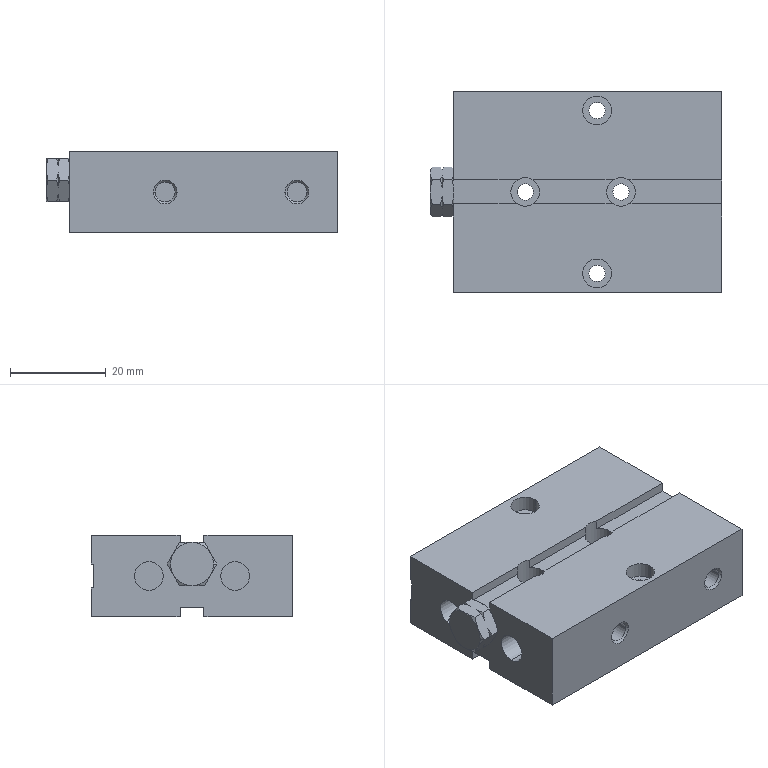Part | SolidWorks | features BaseBody 1 | 1 solid | 114 faces | box 60.8 x 42 x 17 mm | volume 37225 mm3 | plane 50 | cylinder 32 | cone 32 | commonest cylinder face diameters 6 x20 3.4 x8 4.134 x4